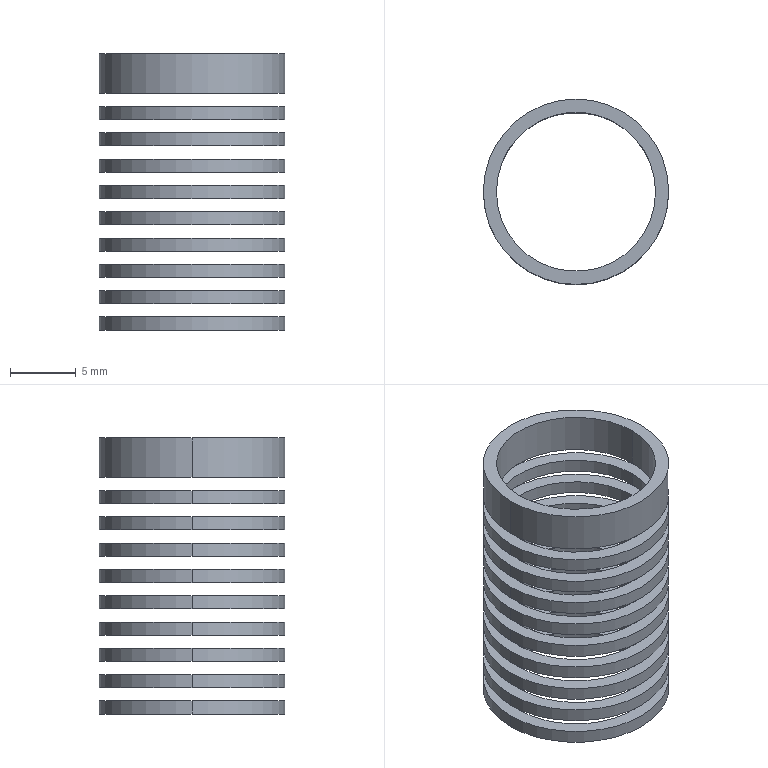Part | STEP file | f5-13-063 | 10 solids | 60 faces | box 14.1 x 14.1 x 21 mm | volume 493.858 mm3 | cylinder 40 | plane 20 | commonest cylinder face diameters 12.1 x20 14.1 x20